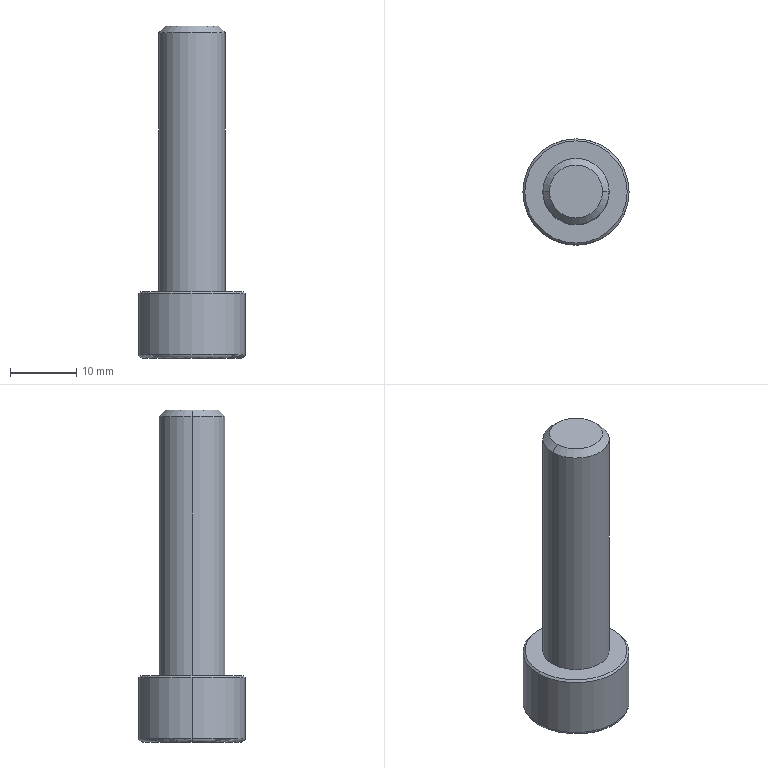Part | NX | features BREP 1 | 1 solid | 20 faces | box 16 x 16 x 50 mm | volume 4800 mm3 | plane 10 | cylinder 4 | cone 4 | torus 2 | commonest cylinder face diameters 10 x2 16 x2
STEP:
#1=CARTESIAN_POINT('',(-7.5,0.,0.));
#2=VERTEX_POINT('',#1);
#3=CARTESIAN_POINT('',(7.5,0.,0.));
#4=VERTEX_POINT('',#3);
#5=CARTESIAN_POINT('',(0.,0.,0.));
#6=DIRECTION('',(0.,0.,-1.));
#7=DIRECTION('',(-1.,0.,0.));
#8=AXIS2_PLACEMENT_3D('',#5,#6,#7);
#9=CIRCLE('',#8,7.5);
#10=EDGE_CURVE('',#2,#4,#9,.T.);
#11=ORIENTED_EDGE('',*,*,#10,.T.);
#12=CARTESIAN_POINT('',(0.,0.,0.));
#13=DIRECTION('',(0.,0.,-1.));
#14=DIRECTION('',(1.,0.,0.));
#15=AXIS2_PLACEMENT_3D('',#12,#13,#14);
#16=CIRCLE('',#15,7.5);
#17=EDGE_CURVE('',#4,#2,#16,.T.);
#18=ORIENTED_EDGE('',*,*,#17,.T.);
#19=EDGE_LOOP('',(#11,#18));
#20=FACE_BOUND('',#19,.T.);
#21=CARTESIAN_POINT('',(0.,-4.619,0.));
#22=VERTEX_POINT('',#21);
#23=CARTESIAN_POINT('',(4.,-2.309,0.));
#24=VERTEX_POINT('',#23);
#25=CARTESIAN_POINT('',(0.,-4.619,0.));
#26=DIRECTION('',(0.866,0.5,0.));
#27=VECTOR('',#26,1000.);
#28=LINE('',#25,#27);
#29=EDGE_CURVE('',#22,#24,#28,.T.);
#30=ORIENTED_EDGE('',*,*,#29,.T.);
#31=CARTESIAN_POINT('',(4.,2.309,0.));
#32=VERTEX_POINT('',#31);
#33=CARTESIAN_POINT('',(4.,-2.309,0.));
#34=DIRECTION('',(0.,1.,0.));
#35=VECTOR('',#34,1000.);
#36=LINE('',#33,#35);
#37=EDGE_CURVE('',#24,#32,#36,.T.);
#38=ORIENTED_EDGE('',*,*,#37,.T.);
#39=CARTESIAN_POINT('',(0.,4.619,0.));
#40=VERTEX_POINT('',#39);
#41=CARTESIAN_POINT('',(4.,2.309,0.));
#42=DIRECTION('',(-0.866,0.5,0.));
#43=VECTOR('',#42,1000.);
#44=LINE('',#41,#43);
#45=EDGE_CURVE('',#32,#40,#44,.T.);
#46=ORIENTED_EDGE('',*,*,#45,.T.);
#47=CARTESIAN_POINT('',(-4.,2.309,0.));
#48=VERTEX_POINT('',#47);
#49=CARTESIAN_POINT('',(0.,4.619,0.));
#50=DIRECTION('',(-0.866,-0.5,0.));
#51=VECTOR('',#50,1000.);
#52=LINE('',#49,#51);
#53=EDGE_CURVE('',#40,#48,#52,.T.);
#54=ORIENTED_EDGE('',*,*,#53,.T.);
#55=CARTESIAN_POINT('',(-4.,-2.309,0.));
#56=VERTEX_POINT('',#55);
#57=CARTESIAN_POINT('',(-4.,2.309,0.));
#58=DIRECTION('',(0.,-1.,0.));
#59=VECTOR('',#58,1000.);
#60=LINE('',#57,#59);
#61=EDGE_CURVE('',#48,#56,#60,.T.);
#62=ORIENTED_EDGE('',*,*,#61,.T.);
#63=CARTESIAN_POINT('',(-4.,-2.309,0.));
#64=DIRECTION('',(0.866,-0.5,0.));
#65=VECTOR('',#64,1000.);
#66=LINE('',#63,#65);
#67=EDGE_CURVE('',#56,#22,#66,.T.);
#68=ORIENTED_EDGE('',*,*,#67,.T.);
#69=EDGE_LOOP('',(#30,#38,#46,#54,#62,#68));
#70=FACE_BOUND('',#69,.T.);
#71=CARTESIAN_POINT('',(0.,0.,0.));
#72=DIRECTION('',(0.,0.,1.));
#73=DIRECTION('',(-1.,0.,0.));
#74=AXIS2_PLACEMENT_3D('',#71,#72,#73);
#75=PLANE('',#74);
#76=ADVANCED_FACE('',(#20,#70),#75,.F.);
#77=ORIENTED_EDGE('',*,*,#17,.F.);
#78=CARTESIAN_POINT('',(8.,0.,0.5));
#79=VERTEX_POINT('',#78);
#80=CARTESIAN_POINT('',(7.5,0.,0.5));
#81=DIRECTION('',(0.,1.,0.));
#82=DIRECTION('',(1.,0.,0.));
#83=AXIS2_PLACEMENT_3D('',#80,#81,#82);
#84=CIRCLE('',#83,0.5);
#85=EDGE_CURVE('',#79,#4,#84,.T.);
#86=ORIENTED_EDGE('',*,*,#85,.F.);
#87=CARTESIAN_POINT('',(-8.,0.,0.5));
#88=VERTEX_POINT('',#87);
#89=CARTESIAN_POINT('',(0.,0.,0.5));
#90=DIRECTION('',(0.,0.,-1.));
#91=DIRECTION('',(1.,0.,0.));
#92=AXIS2_PLACEMENT_3D('',#89,#90,#91);
#93=CIRCLE('',#92,8.);
#94=EDGE_CURVE('',#79,#88,#93,.T.);
#95=ORIENTED_EDGE('',*,*,#94,.T.);
#96=CARTESIAN_POINT('',(-7.5,0.,0.5));
#97=DIRECTION('',(0.,-1.,0.));
#98=DIRECTION('',(-1.,0.,0.));
#99=AXIS2_PLACEMENT_3D('',#96,#97,#98);
#100=CIRCLE('',#99,0.5);
#101=EDGE_CURVE('',#88,#2,#100,.T.);
#102=ORIENTED_EDGE('',*,*,#101,.T.);
#103=EDGE_LOOP('',(#77,#86,#95,#102));
#104=FACE_BOUND('',#103,.T.);
#105=CARTESIAN_POINT('',(0.,0.,0.5));
#106=DIRECTION('',(0.,0.,1.));
#107=DIRECTION('',(-1.,0.,0.));
#108=AXIS2_PLACEMENT_3D('',#105,#106,#107);
#109=TOROIDAL_SURFACE('',#108,7.5,0.5);
#110=ADVANCED_FACE('',(#104),#109,.T.);
#111=ORIENTED_EDGE('',*,*,#101,.F.);
#112=CARTESIAN_POINT('',(0.,0.,0.5));
#113=DIRECTION('',(0.,0.,-1.));
#114=DIRECTION('',(-1.,0.,0.));
#115=AXIS2_PLACEMENT_3D('',#112,#113,#114);
#116=CIRCLE('',#115,8.);
#117=EDGE_CURVE('',#88,#79,#116,.T.);
#118=ORIENTED_EDGE('',*,*,#117,.T.);
#119=ORIENTED_EDGE('',*,*,#85,.T.);
#120=ORIENTED_EDGE('',*,*,#10,.F.);
#121=EDGE_LOOP('',(#111,#118,#119,#120));
#122=FACE_BOUND('',#121,.T.);
#123=CARTESIAN_POINT('',(0.,0.,0.5));
#124=DIRECTION('',(0.,0.,1.));
#125=DIRECTION('',(-1.,0.,0.));
#126=AXIS2_PLACEMENT_3D('',#123,#124,#125);
#127=TOROIDAL_SURFACE('',#126,7.5,0.5);
#128=ADVANCED_FACE('',(#122),#127,.T.);
#129=CARTESIAN_POINT('',(8.,0.,9.7));
#130=VERTEX_POINT('',#129);
#131=CARTESIAN_POINT('',(8.,0.,0.5));
#132=DIRECTION('',(0.,0.,1.));
#133=VECTOR('',#132,1000.);
#134=LINE('',#131,#133);
#135=EDGE_CURVE('',#79,#130,#134,.T.);
#136=ORIENTED_EDGE('',*,*,#135,.F.);
#137=ORIENTED_EDGE('',*,*,#117,.F.);
#138=CARTESIAN_POINT('',(-8.,0.,9.7));
#139=VERTEX_POINT('',#138);
#140=CARTESIAN_POINT('',(-8.,0.,0.5));
#141=DIRECTION('',(0.,0.,1.));
#142=VECTOR('',#141,1000.);
#143=LINE('',#140,#142);
#144=EDGE_CURVE('',#88,#139,#143,.T.);
#145=ORIENTED_EDGE('',*,*,#144,.T.);
#146=CARTESIAN_POINT('',(0.,0.,9.7));
#147=DIRECTION('',(0.,0.,1.));
#148=DIRECTION('',(1.,0.,0.));
#149=AXIS2_PLACEMENT_3D('',#146,#147,#148);
#150=CIRCLE('',#149,8.);
#151=EDGE_CURVE('',#130,#139,#150,.T.);
#152=ORIENTED_EDGE('',*,*,#151,.F.);
#153=EDGE_LOOP('',(#136,#137,#145,#152));
#154=FACE_BOUND('',#153,.T.);
#155=CARTESIAN_POINT('',(0.,0.,10.));
#156=DIRECTION('',(0.,0.,-1.));
#157=DIRECTION('',(1.,0.,0.));
#158=AXIS2_PLACEMENT_3D('',#155,#156,#157);
#159=CYLINDRICAL_SURFACE('',#158,8.);
#160=ADVANCED_FACE('',(#154),#159,.T.);
#161=CARTESIAN_POINT('',(7.7,0.,10.));
#162=VERTEX_POINT('',#161);
#163=CARTESIAN_POINT('',(8.,0.,9.7));
#164=DIRECTION('',(-0.7071,0.,0.7071));
#165=VECTOR('',#164,1000.);
#166=LINE('',#163,#165);
#167=EDGE_CURVE('',#130,#162,#166,.T.);
#168=ORIENTED_EDGE('',*,*,#167,.F.);
#169=ORIENTED_EDGE('',*,*,#151,.T.);
#170=CARTESIAN_POINT('',(-7.7,0.,10.));
#171=VERTEX_POINT('',#170);
#172=CARTESIAN_POINT('',(-8.,0.,9.7));
#173=DIRECTION('',(0.7071,0.,0.7071));
#174=VECTOR('',#173,1000.);
#175=LINE('',#172,#174);
#176=EDGE_CURVE('',#139,#171,#175,.T.);
#177=ORIENTED_EDGE('',*,*,#176,.T.);
#178=CARTESIAN_POINT('',(0.,0.,10.));
#179=DIRECTION('',(0.,0.,1.));
#180=DIRECTION('',(1.,0.,0.));
#181=AXIS2_PLACEMENT_3D('',#178,#179,#180);
#182=CIRCLE('',#181,7.7);
#183=EDGE_CURVE('',#162,#171,#182,.T.);
#184=ORIENTED_EDGE('',*,*,#183,.F.);
#185=EDGE_LOOP('',(#168,#169,#177,#184));
#186=FACE_BOUND('',#185,.T.);
#187=CARTESIAN_POINT('',(0.,0.,9.85));
#188=DIRECTION('',(0.,0.,-1.));
#189=DIRECTION('',(1.,0.,0.));
#190=AXIS2_PLACEMENT_3D('',#187,#188,#189);
#191=CONICAL_SURFACE('',#190,7.85,0.7854);
#192=ADVANCED_FACE('',(#186),#191,.T.);
#193=ORIENTED_EDGE('',*,*,#183,.T.);
#194=CARTESIAN_POINT('',(0.,0.,10.));
#195=DIRECTION('',(0.,0.,1.));
#196=DIRECTION('',(-1.,0.,0.));
#197=AXIS2_PLACEMENT_3D('',#194,#195,#196);
#198=CIRCLE('',#197,7.7);
#199=EDGE_CURVE('',#171,#162,#198,.T.);
#200=ORIENTED_EDGE('',*,*,#199,.T.);
#201=EDGE_LOOP('',(#193,#200));
#202=FACE_BOUND('',#201,.T.);
#203=CARTESIAN_POINT('',(-5.,0.,10.));
#204=VERTEX_POINT('',#203);
#205=CARTESIAN_POINT('',(5.,0.,10.));
#206=VERTEX_POINT('',#205);
#207=CARTESIAN_POINT('',(0.,0.,10.));
#208=DIRECTION('',(0.,0.,-1.));
#209=DIRECTION('',(-1.,0.,0.));
#210=AXIS2_PLACEMENT_3D('',#207,#208,#209);
#211=CIRCLE('',#210,5.);
#212=EDGE_CURVE('',#204,#206,#211,.T.);
#213=ORIENTED_EDGE('',*,*,#212,.T.);
#214=CARTESIAN_POINT('',(0.,0.,10.));
#215=DIRECTION('',(0.,0.,-1.));
#216=DIRECTION('',(1.,0.,0.));
#217=AXIS2_PLACEMENT_3D('',#214,#215,#216);
#218=CIRCLE('',#217,5.);
#219=EDGE_CURVE('',#206,#204,#218,.T.);
#220=ORIENTED_EDGE('',*,*,#219,.T.);
#221=EDGE_LOOP('',(#213,#220));
#222=FACE_BOUND('',#221,.T.);
#223=CARTESIAN_POINT('',(0.,0.,10.));
#224=DIRECTION('',(0.,0.,1.));
#225=DIRECTION('',(-1.,0.,0.));
#226=AXIS2_PLACEMENT_3D('',#223,#224,#225);
#227=PLANE('',#226);
#228=ADVANCED_FACE('',(#202,#222),#227,.T.);
#229=ORIENTED_EDGE('',*,*,#199,.F.);
#230=ORIENTED_EDGE('',*,*,#176,.F.);
#231=CARTESIAN_POINT('',(0.,0.,9.7));
#232=DIRECTION('',(0.,0.,1.));
#233=DIRECTION('',(-1.,0.,0.));
#234=AXIS2_PLACEMENT_3D('',#231,#232,#233);
#235=CIRCLE('',#234,8.);
#236=EDGE_CURVE('',#139,#130,#235,.T.);
#237=ORIENTED_EDGE('',*,*,#236,.T.);
#238=ORIENTED_EDGE('',*,*,#167,.T.);
#239=EDGE_LOOP('',(#229,#230,#237,#238));
#240=FACE_BOUND('',#239,.T.);
#241=CARTESIAN_POINT('',(0.,0.,9.85));
#242=DIRECTION('',(0.,0.,-1.));
#243=DIRECTION('',(1.,0.,0.));
#244=AXIS2_PLACEMENT_3D('',#241,#242,#243);
#245=CONICAL_SURFACE('',#244,7.85,0.7854);
#246=ADVANCED_FACE('',(#240),#245,.T.);
#247=ORIENTED_EDGE('',*,*,#236,.F.);
#248=ORIENTED_EDGE('',*,*,#144,.F.);
#249=ORIENTED_EDGE('',*,*,#94,.F.);
#250=ORIENTED_EDGE('',*,*,#135,.T.);
#251=EDGE_LOOP('',(#247,#248,#249,#250));
#252=FACE_BOUND('',#251,.T.);
#253=CARTESIAN_POINT('',(0.,0.,10.));
#254=DIRECTION('',(0.,0.,-1.));
#255=DIRECTION('',(1.,0.,0.));
#256=AXIS2_PLACEMENT_3D('',#253,#254,#255);
#257=CYLINDRICAL_SURFACE('',#256,8.);
#258=ADVANCED_FACE('',(#252),#257,.T.);
#259=CARTESIAN_POINT('',(-5.,0.,49.));
#260=VERTEX_POINT('',#259);
#261=CARTESIAN_POINT('',(5.,0.,49.));
#262=VERTEX_POINT('',#261);
#263=CARTESIAN_POINT('',(0.,0.,49.));
#264=DIRECTION('',(0.,0.,1.));
#265=DIRECTION('',(-1.,0.,0.));
#266=AXIS2_PLACEMENT_3D('',#263,#264,#265);
#267=CIRCLE('',#266,5.);
#268=EDGE_CURVE('',#260,#262,#267,.T.);
#269=ORIENTED_EDGE('',*,*,#268,.F.);
#270=CARTESIAN_POINT('',(-5.,0.,10.));
#271=DIRECTION('',(0.,0.,1.));
#272=VECTOR('',#271,1000.);
#273=LINE('',#270,#272);
#274=EDGE_CURVE('',#260,#204,#273,.F.);
#275=ORIENTED_EDGE('',*,*,#274,.T.);
#276=ORIENTED_EDGE('',*,*,#219,.F.);
#277=CARTESIAN_POINT('',(5.,0.,10.));
#278=DIRECTION('',(0.,0.,1.));
#279=VECTOR('',#278,1000.);
#280=LINE('',#277,#279);
#281=EDGE_CURVE('',#262,#206,#280,.F.);
#282=ORIENTED_EDGE('',*,*,#281,.F.);
#283=EDGE_LOOP('',(#269,#275,#276,#282));
#284=FACE_BOUND('',#283,.T.);
#285=CARTESIAN_POINT('',(0.,0.,50.));
#286=DIRECTION('',(0.,0.,-1.));
#287=DIRECTION('',(1.,0.,0.));
#288=AXIS2_PLACEMENT_3D('',#285,#286,#287);
#289=CYLINDRICAL_SURFACE('',#288,5.);
#290=ADVANCED_FACE('',(#284),#289,.T.);
#291=ORIENTED_EDGE('',*,*,#281,.T.);
#292=ORIENTED_EDGE('',*,*,#212,.F.);
#293=ORIENTED_EDGE('',*,*,#274,.F.);
#294=CARTESIAN_POINT('',(0.,0.,49.));
#295=DIRECTION('',(0.,0.,1.));
#296=DIRECTION('',(1.,0.,0.));
#297=AXIS2_PLACEMENT_3D('',#294,#295,#296);
#298=CIRCLE('',#297,5.);
#299=EDGE_CURVE('',#262,#260,#298,.T.);
#300=ORIENTED_EDGE('',*,*,#299,.F.);
#301=EDGE_LOOP('',(#291,#292,#293,#300));
#302=FACE_BOUND('',#301,.T.);
#303=CARTESIAN_POINT('',(0.,0.,50.));
#304=DIRECTION('',(0.,0.,-1.));
#305=DIRECTION('',(1.,0.,0.));
#306=AXIS2_PLACEMENT_3D('',#303,#304,#305);
#307=CYLINDRICAL_SURFACE('',#306,5.);
#308=ADVANCED_FACE('',(#302),#307,.T.);
#309=CARTESIAN_POINT('',(4.,0.,50.));
#310=VERTEX_POINT('',#309);
#311=CARTESIAN_POINT('',(5.,0.,49.));
#312=DIRECTION('',(-0.7071,0.,0.7071));
#313=VECTOR('',#312,1000.);
#314=LINE('',#311,#313);
#315=EDGE_CURVE('',#262,#310,#314,.T.);
#316=ORIENTED_EDGE('',*,*,#315,.F.);
#317=ORIENTED_EDGE('',*,*,#299,.T.);
#318=CARTESIAN_POINT('',(-4.,0.,50.));
#319=VERTEX_POINT('',#318);
#320=CARTESIAN_POINT('',(-5.,0.,49.));
#321=DIRECTION('',(0.7071,0.,0.7071));
#322=VECTOR('',#321,1000.);
#323=LINE('',#320,#322);
#324=EDGE_CURVE('',#260,#319,#323,.T.);
#325=ORIENTED_EDGE('',*,*,#324,.T.);
#326=CARTESIAN_POINT('',(0.,0.,50.));
#327=DIRECTION('',(0.,0.,1.));
#328=DIRECTION('',(1.,0.,0.));
#329=AXIS2_PLACEMENT_3D('',#326,#327,#328);
#330=CIRCLE('',#329,4.);
#331=EDGE_CURVE('',#310,#319,#330,.T.);
#332=ORIENTED_EDGE('',*,*,#331,.F.);
#333=EDGE_LOOP('',(#316,#317,#325,#332));
#334=FACE_BOUND('',#333,.T.);
#335=CARTESIAN_POINT('',(0.,0.,49.5));
#336=DIRECTION('',(0.,0.,-1.));
#337=DIRECTION('',(1.,0.,0.));
#338=AXIS2_PLACEMENT_3D('',#335,#336,#337);
#339=CONICAL_SURFACE('',#338,4.5,0.7854);
#340=ADVANCED_FACE('',(#334),#339,.T.);
#341=ORIENTED_EDGE('',*,*,#331,.T.);
#342=CARTESIAN_POINT('',(0.,0.,50.));
#343=DIRECTION('',(0.,0.,1.));
#344=DIRECTION('',(-1.,0.,0.));
#345=AXIS2_PLACEMENT_3D('',#342,#343,#344);
#346=CIRCLE('',#345,4.);
#347=EDGE_CURVE('',#319,#310,#346,.T.);
#348=ORIENTED_EDGE('',*,*,#347,.T.);
#349=EDGE_LOOP('',(#341,#348));
#350=FACE_BOUND('',#349,.T.);
#351=CARTESIAN_POINT('',(0.,0.,50.));
#352=DIRECTION('',(0.,0.,1.));
#353=DIRECTION('',(-1.,0.,0.));
#354=AXIS2_PLACEMENT_3D('',#351,#352,#353);
#355=PLANE('',#354);
#356=ADVANCED_FACE('',(#350),#355,.T.);
#357=ORIENTED_EDGE('',*,*,#347,.F.);
#358=ORIENTED_EDGE('',*,*,#324,.F.);
#359=ORIENTED_EDGE('',*,*,#268,.T.);
#360=ORIENTED_EDGE('',*,*,#315,.T.);
#361=EDGE_LOOP('',(#357,#358,#359,#360));
#362=FACE_BOUND('',#361,.T.);
#363=CARTESIAN_POINT('',(0.,0.,49.5));
#364=DIRECTION('',(0.,0.,-1.));
#365=DIRECTION('',(1.,0.,0.));
#366=AXIS2_PLACEMENT_3D('',#363,#364,#365);
#367=CONICAL_SURFACE('',#366,4.5,0.7854);
#368=ADVANCED_FACE('',(#362),#367,.T.);
#369=CARTESIAN_POINT('',(-4.,-2.309,6.));
#370=VERTEX_POINT('',#369);
#371=CARTESIAN_POINT('',(-4.,-2.309,0.));
#372=DIRECTION('',(0.,0.,1.));
#373=VECTOR('',#372,1000.);
#374=LINE('',#371,#373);
#375=EDGE_CURVE('',#56,#370,#374,.T.);
#376=ORIENTED_EDGE('',*,*,#375,.T.);
#377=CARTESIAN_POINT('',(0.,-4.619,6.));
#378=VERTEX_POINT('',#377);
#379=CARTESIAN_POINT('',(0.,-4.619,6.));
#380=DIRECTION('',(-0.866,0.5,0.));
#381=VECTOR('',#380,1000.);
#382=LINE('',#379,#381);
#383=EDGE_CURVE('',#378,#370,#382,.T.);
#384=ORIENTED_EDGE('',*,*,#383,.F.);
#385=CARTESIAN_POINT('',(0.,-4.619,0.));
#386=DIRECTION('',(0.,0.,1.));
#387=VECTOR('',#386,1000.);
#388=LINE('',#385,#387);
#389=EDGE_CURVE('',#22,#378,#388,.T.);
#390=ORIENTED_EDGE('',*,*,#389,.F.);
#391=ORIENTED_EDGE('',*,*,#67,.F.);
#392=EDGE_LOOP('',(#376,#384,#390,#391));
#393=FACE_BOUND('',#392,.T.);
#394=CARTESIAN_POINT('',(0.,-4.619,6.));
#395=DIRECTION('',(-0.5,-0.866,0.));
#396=DIRECTION('',(-0.866,0.5,0.));
#397=AXIS2_PLACEMENT_3D('',#394,#395,#396);
#398=PLANE('',#397);
#399=ADVANCED_FACE('',(#393),#398,.F.);
#400=ORIENTED_EDGE('',*,*,#389,.T.);
#401=CARTESIAN_POINT('',(4.,-2.309,6.));
#402=VERTEX_POINT('',#401);
#403=CARTESIAN_POINT('',(4.,-2.309,6.));
#404=DIRECTION('',(-0.866,-0.5,0.));
#405=VECTOR('',#404,1000.);
#406=LINE('',#403,#405);
#407=EDGE_CURVE('',#402,#378,#406,.T.);
#408=ORIENTED_EDGE('',*,*,#407,.F.);
#409=CARTESIAN_POINT('',(4.,-2.309,0.));
#410=DIRECTION('',(0.,0.,1.));
#411=VECTOR('',#410,1000.);
#412=LINE('',#409,#411);
#413=EDGE_CURVE('',#24,#402,#412,.T.);
#414=ORIENTED_EDGE('',*,*,#413,.F.);
#415=ORIENTED_EDGE('',*,*,#29,.F.);
#416=EDGE_LOOP('',(#400,#408,#414,#415));
#417=FACE_BOUND('',#416,.T.);
#418=CARTESIAN_POINT('',(4.,-2.309,6.));
#419=DIRECTION('',(0.5,-0.866,0.));
#420=DIRECTION('',(-0.866,-0.5,0.));
#421=AXIS2_PLACEMENT_3D('',#418,#419,#420);
#422=PLANE('',#421);
#423=ADVANCED_FACE('',(#417),#422,.F.);
#424=ORIENTED_EDGE('',*,*,#413,.T.);
#425=CARTESIAN_POINT('',(4.,2.309,6.));
#426=VERTEX_POINT('',#425);
#427=CARTESIAN_POINT('',(4.,-2.309,6.));
#428=DIRECTION('',(0.,1.,0.));
#429=VECTOR('',#428,1000.);
#430=LINE('',#427,#429);
#431=EDGE_CURVE('',#402,#426,#430,.T.);
#432=ORIENTED_EDGE('',*,*,#431,.T.);
#433=CARTESIAN_POINT('',(4.,2.309,0.));
#434=DIRECTION('',(0.,0.,1.));
#435=VECTOR('',#434,1000.);
#436=LINE('',#433,#435);
#437=EDGE_CURVE('',#32,#426,#436,.T.);
#438=ORIENTED_EDGE('',*,*,#437,.F.);
#439=ORIENTED_EDGE('',*,*,#37,.F.);
#440=EDGE_LOOP('',(#424,#432,#438,#439));
#441=FACE_BOUND('',#440,.T.);
#442=CARTESIAN_POINT('',(4.,2.309,6.));
#443=DIRECTION('',(1.,0.,0.));
#444=DIRECTION('',(0.,0.,1.));
#445=AXIS2_PLACEMENT_3D('',#442,#443,#444);
#446=PLANE('',#445);
#447=ADVANCED_FACE('',(#441),#446,.F.);
#448=ORIENTED_EDGE('',*,*,#437,.T.);
#449=CARTESIAN_POINT('',(0.,4.619,6.));
#450=VERTEX_POINT('',#449);
#451=CARTESIAN_POINT('',(0.,4.619,6.));
#452=DIRECTION('',(0.866,-0.5,0.));
#453=VECTOR('',#452,1000.);
#454=LINE('',#451,#453);
#455=EDGE_CURVE('',#450,#426,#454,.T.);
#456=ORIENTED_EDGE('',*,*,#455,.F.);
#457=CARTESIAN_POINT('',(0.,4.619,0.));
#458=DIRECTION('',(0.,0.,1.));
#459=VECTOR('',#458,1000.);
#460=LINE('',#457,#459);
#461=EDGE_CURVE('',#40,#450,#460,.T.);
#462=ORIENTED_EDGE('',*,*,#461,.F.);
#463=ORIENTED_EDGE('',*,*,#45,.F.);
#464=EDGE_LOOP('',(#448,#456,#462,#463));
#465=FACE_BOUND('',#464,.T.);
#466=CARTESIAN_POINT('',(0.,4.619,6.));
#467=DIRECTION('',(0.5,0.866,0.));
#468=DIRECTION('',(0.866,-0.5,0.));
#469=AXIS2_PLACEMENT_3D('',#466,#467,#468);
#470=PLANE('',#469);
#471=ADVANCED_FACE('',(#465),#470,.F.);
#472=ORIENTED_EDGE('',*,*,#461,.T.);
#473=CARTESIAN_POINT('',(-4.,2.309,6.));
#474=VERTEX_POINT('',#473);
#475=CARTESIAN_POINT('',(-4.,2.309,6.));
#476=DIRECTION('',(0.866,0.5,0.));
#477=VECTOR('',#476,1000.);
#478=LINE('',#475,#477);
#479=EDGE_CURVE('',#474,#450,#478,.T.);
#480=ORIENTED_EDGE('',*,*,#479,.F.);
#481=CARTESIAN_POINT('',(-4.,2.309,0.));
#482=DIRECTION('',(0.,0.,1.));
#483=VECTOR('',#482,1000.);
#484=LINE('',#481,#483);
#485=EDGE_CURVE('',#48,#474,#484,.T.);
#486=ORIENTED_EDGE('',*,*,#485,.F.);
#487=ORIENTED_EDGE('',*,*,#53,.F.);
#488=EDGE_LOOP('',(#472,#480,#486,#487));
#489=FACE_BOUND('',#488,.T.);
#490=CARTESIAN_POINT('',(-4.,2.309,6.));
#491=DIRECTION('',(-0.5,0.866,0.));
#492=DIRECTION('',(0.866,0.5,0.));
#493=AXIS2_PLACEMENT_3D('',#490,#491,#492);
#494=PLANE('',#493);
#495=ADVANCED_FACE('',(#489),#494,.F.);
#496=ORIENTED_EDGE('',*,*,#485,.T.);
#497=CARTESIAN_POINT('',(-4.,2.309,6.));
#498=DIRECTION('',(0.,-1.,0.));
#499=VECTOR('',#498,1000.);
#500=LINE('',#497,#499);
#501=EDGE_CURVE('',#474,#370,#500,.T.);
#502=ORIENTED_EDGE('',*,*,#501,.T.);
#503=ORIENTED_EDGE('',*,*,#375,.F.);
#504=ORIENTED_EDGE('',*,*,#61,.F.);
#505=EDGE_LOOP('',(#496,#502,#503,#504));
#506=FACE_BOUND('',#505,.T.);
#507=CARTESIAN_POINT('',(-4.,-2.309,6.));
#508=DIRECTION('',(-1.,0.,0.));
#509=DIRECTION('',(0.,0.,-1.));
#510=AXIS2_PLACEMENT_3D('',#507,#508,#509);
#511=PLANE('',#510);
#512=ADVANCED_FACE('',(#506),#511,.F.);
#513=ORIENTED_EDGE('',*,*,#383,.T.);
#514=ORIENTED_EDGE('',*,*,#501,.F.);
#515=ORIENTED_EDGE('',*,*,#479,.T.);
#516=ORIENTED_EDGE('',*,*,#455,.T.);
#517=ORIENTED_EDGE('',*,*,#431,.F.);
#518=ORIENTED_EDGE('',*,*,#407,.T.);
#519=EDGE_LOOP('',(#513,#514,#515,#516,#517,#518));
#520=FACE_BOUND('',#519,.T.);
#521=CARTESIAN_POINT('',(0.,0.,6.));
#522=DIRECTION('',(0.,0.,-1.));
#523=DIRECTION('',(1.,0.,0.));
#524=AXIS2_PLACEMENT_3D('',#521,#522,#523);
#525=PLANE('',#524);
#526=ADVANCED_FACE('',(#520),#525,.T.);
#527=CLOSED_SHELL('',(#76,#110,#128,#160,#192,#228,#246,#258,#290,#308,#340,#356,#368,#399,#423,#447,#471,#495,#512,#526));
#528=MANIFOLD_SOLID_BREP('',#527);
#529=(LENGTH_UNIT()NAMED_UNIT(*)SI_UNIT(.MILLI.,.METRE.));
#530=UNCERTAINTY_MEASURE_WITH_UNIT(LENGTH_MEASURE(0.00001),#529,'','');
#531=(NAMED_UNIT(*)PLANE_ANGLE_UNIT()SI_UNIT($,.RADIAN.));
#532=(NAMED_UNIT(*)SI_UNIT($,.STERADIAN.)SOLID_ANGLE_UNIT());
#533=(GEOMETRIC_REPRESENTATION_CONTEXT(3)GLOBAL_UNCERTAINTY_ASSIGNED_CONTEXT((#530))GLOBAL_UNIT_ASSIGNED_CONTEXT((#529,#531,#532))REPRESENTATION_CONTEXT('',''));
#534=ADVANCED_BREP_SHAPE_REPRESENTATION('',(#528),#533);